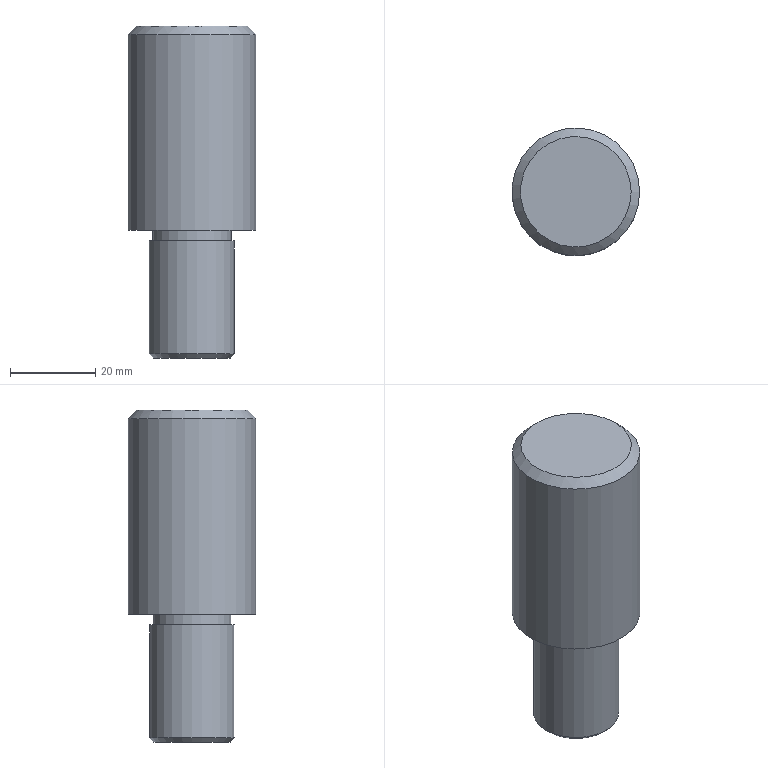Part | NX | features CYLINDER 3, CHAMFER 2, DATUM_CSYS 1 | 1 solid | 9 faces | box 30 x 30 x 78 mm | volume 43030 mm3 | plane 4 | cylinder 3 | cone 2 | commonest cylinder face diameters 18.5 x1 20 x1 30 x1
STEP:
#1=CARTESIAN_POINT('',(13.,0.,48.));
#2=VERTEX_POINT('',#1);
#3=CARTESIAN_POINT('',(0.,0.,48.));
#4=DIRECTION('',(0.,0.,1.));
#5=DIRECTION('',(1.,0.,0.));
#6=AXIS2_PLACEMENT_3D('',#3,#4,#5);
#7=CIRCLE('',#6,13.);
#8=EDGE_CURVE('',#2,#2,#7,.T.);
#9=ORIENTED_EDGE('',*,*,#8,.T.);
#10=EDGE_LOOP('',(#9));
#11=FACE_BOUND('',#10,.T.);
#12=CARTESIAN_POINT('',(0.,0.,48.));
#13=DIRECTION('',(0.,0.,1.));
#14=DIRECTION('',(1.,0.,0.));
#15=AXIS2_PLACEMENT_3D('',#12,#13,#14);
#16=PLANE('',#15);
#17=ADVANCED_FACE('',(#11),#16,.T.);
#18=CARTESIAN_POINT('',(9.25,0.,0.));
#19=VERTEX_POINT('',#18);
#20=CARTESIAN_POINT('',(0.,0.,0.));
#21=DIRECTION('',(0.,0.,-1.));
#22=DIRECTION('',(1.,0.,0.));
#23=AXIS2_PLACEMENT_3D('',#20,#21,#22);
#24=CIRCLE('',#23,9.25);
#25=EDGE_CURVE('',#19,#19,#24,.T.);
#26=ORIENTED_EDGE('',*,*,#25,.F.);
#27=EDGE_LOOP('',(#26));
#28=FACE_BOUND('',#27,.T.);
#29=CARTESIAN_POINT('',(15.,0.,0.));
#30=VERTEX_POINT('',#29);
#31=CARTESIAN_POINT('',(0.,0.,0.));
#32=DIRECTION('',(0.,0.,1.));
#33=DIRECTION('',(1.,0.,0.));
#34=AXIS2_PLACEMENT_3D('',#31,#32,#33);
#35=CIRCLE('',#34,15.);
#36=EDGE_CURVE('',#30,#30,#35,.T.);
#37=ORIENTED_EDGE('',*,*,#36,.F.);
#38=EDGE_LOOP('',(#37));
#39=FACE_BOUND('',#38,.T.);
#40=CARTESIAN_POINT('',(0.,0.,0.));
#41=DIRECTION('',(0.,0.,-1.));
#42=DIRECTION('',(-1.,0.,0.));
#43=AXIS2_PLACEMENT_3D('',#40,#41,#42);
#44=PLANE('',#43);
#45=ADVANCED_FACE('',(#28,#39),#44,.T.);
#46=CARTESIAN_POINT('',(15.,0.,46.));
#47=VERTEX_POINT('',#46);
#48=CARTESIAN_POINT('',(0.,0.,46.));
#49=DIRECTION('',(0.,0.,1.));
#50=DIRECTION('',(1.,0.,0.));
#51=AXIS2_PLACEMENT_3D('',#48,#49,#50);
#52=CIRCLE('',#51,15.);
#53=EDGE_CURVE('',#47,#47,#52,.F.);
#54=ORIENTED_EDGE('',*,*,#53,.T.);
#55=EDGE_LOOP('',(#54));
#56=FACE_BOUND('',#55,.T.);
#57=ORIENTED_EDGE('',*,*,#36,.T.);
#58=EDGE_LOOP('',(#57));
#59=FACE_BOUND('',#58,.T.);
#60=CARTESIAN_POINT('',(0.,0.,0.));
#61=DIRECTION('',(0.,0.,1.));
#62=DIRECTION('',(1.,0.,0.));
#63=AXIS2_PLACEMENT_3D('',#60,#61,#62);
#64=CYLINDRICAL_SURFACE('',#63,15.);
#65=ADVANCED_FACE('',(#56,#59),#64,.T.);
#66=CARTESIAN_POINT('',(9.25,0.,-2.5));
#67=VERTEX_POINT('',#66);
#68=CARTESIAN_POINT('',(0.,0.,-2.5));
#69=DIRECTION('',(0.,0.,1.));
#70=DIRECTION('',(1.,0.,0.));
#71=AXIS2_PLACEMENT_3D('',#68,#69,#70);
#72=CIRCLE('',#71,9.25);
#73=EDGE_CURVE('',#67,#67,#72,.T.);
#74=ORIENTED_EDGE('',*,*,#73,.T.);
#75=EDGE_LOOP('',(#74));
#76=FACE_BOUND('',#75,.T.);
#77=ORIENTED_EDGE('',*,*,#25,.T.);
#78=EDGE_LOOP('',(#77));
#79=FACE_BOUND('',#78,.T.);
#80=CARTESIAN_POINT('',(0.,0.,0.));
#81=DIRECTION('',(0.,0.,-1.));
#82=DIRECTION('',(1.,0.,0.));
#83=AXIS2_PLACEMENT_3D('',#80,#81,#82);
#84=CYLINDRICAL_SURFACE('',#83,9.25);
#85=ADVANCED_FACE('',(#76,#79),#84,.T.);
#86=CARTESIAN_POINT('',(-9.,0.,-30.));
#87=VERTEX_POINT('',#86);
#88=CARTESIAN_POINT('',(0.,0.,-30.));
#89=DIRECTION('',(0.,0.,-1.));
#90=DIRECTION('',(-1.,0.,0.));
#91=AXIS2_PLACEMENT_3D('',#88,#89,#90);
#92=CIRCLE('',#91,9.);
#93=EDGE_CURVE('',#87,#87,#92,.T.);
#94=ORIENTED_EDGE('',*,*,#93,.T.);
#95=EDGE_LOOP('',(#94));
#96=FACE_BOUND('',#95,.T.);
#97=CARTESIAN_POINT('',(0.,0.,-30.));
#98=DIRECTION('',(0.,0.,-1.));
#99=DIRECTION('',(-1.,0.,0.));
#100=AXIS2_PLACEMENT_3D('',#97,#98,#99);
#101=PLANE('',#100);
#102=ADVANCED_FACE('',(#96),#101,.T.);
#103=ORIENTED_EDGE('',*,*,#73,.F.);
#104=EDGE_LOOP('',(#103));
#105=FACE_BOUND('',#104,.T.);
#106=CARTESIAN_POINT('',(10.,0.,-2.5));
#107=VERTEX_POINT('',#106);
#108=CARTESIAN_POINT('',(0.,0.,-2.5));
#109=DIRECTION('',(0.,0.,-1.));
#110=DIRECTION('',(1.,0.,0.));
#111=AXIS2_PLACEMENT_3D('',#108,#109,#110);
#112=CIRCLE('',#111,10.);
#113=EDGE_CURVE('',#107,#107,#112,.T.);
#114=ORIENTED_EDGE('',*,*,#113,.F.);
#115=EDGE_LOOP('',(#114));
#116=FACE_BOUND('',#115,.T.);
#117=CARTESIAN_POINT('',(0.,0.,-2.5));
#118=DIRECTION('',(0.,0.,1.));
#119=DIRECTION('',(1.,0.,0.));
#120=AXIS2_PLACEMENT_3D('',#117,#118,#119);
#121=PLANE('',#120);
#122=ADVANCED_FACE('',(#105,#116),#121,.T.);
#123=CARTESIAN_POINT('',(-10.,0.,-29.));
#124=VERTEX_POINT('',#123);
#125=CARTESIAN_POINT('',(0.,0.,-29.));
#126=DIRECTION('',(0.,0.,-1.));
#127=DIRECTION('',(-1.,0.,0.));
#128=AXIS2_PLACEMENT_3D('',#125,#126,#127);
#129=CIRCLE('',#128,10.);
#130=EDGE_CURVE('',#124,#124,#129,.F.);
#131=ORIENTED_EDGE('',*,*,#130,.T.);
#132=EDGE_LOOP('',(#131));
#133=FACE_BOUND('',#132,.T.);
#134=ORIENTED_EDGE('',*,*,#113,.T.);
#135=EDGE_LOOP('',(#134));
#136=FACE_BOUND('',#135,.T.);
#137=CARTESIAN_POINT('',(0.,0.,-2.5));
#138=DIRECTION('',(0.,0.,-1.));
#139=DIRECTION('',(1.,0.,0.));
#140=AXIS2_PLACEMENT_3D('',#137,#138,#139);
#141=CYLINDRICAL_SURFACE('',#140,10.);
#142=ADVANCED_FACE('',(#133,#136),#141,.T.);
#143=ORIENTED_EDGE('',*,*,#8,.F.);
#144=EDGE_LOOP('',(#143));
#145=FACE_BOUND('',#144,.T.);
#146=ORIENTED_EDGE('',*,*,#53,.F.);
#147=EDGE_LOOP('',(#146));
#148=FACE_BOUND('',#147,.T.);
#149=CARTESIAN_POINT('',(0.,0.,46.));
#150=DIRECTION('',(0.,0.,-1.));
#151=DIRECTION('',(-1.,0.,0.));
#152=AXIS2_PLACEMENT_3D('',#149,#150,#151);
#153=CONICAL_SURFACE('',#152,15.,0.7854);
#154=ADVANCED_FACE('',(#145,#148),#153,.T.);
#155=ORIENTED_EDGE('',*,*,#93,.F.);
#156=EDGE_LOOP('',(#155));
#157=FACE_BOUND('',#156,.T.);
#158=ORIENTED_EDGE('',*,*,#130,.F.);
#159=EDGE_LOOP('',(#158));
#160=FACE_BOUND('',#159,.T.);
#161=CARTESIAN_POINT('',(0.,0.,-29.));
#162=DIRECTION('',(0.,0.,1.));
#163=DIRECTION('',(1.,0.,0.));
#164=AXIS2_PLACEMENT_3D('',#161,#162,#163);
#165=CONICAL_SURFACE('',#164,10.,0.7854);
#166=ADVANCED_FACE('',(#157,#160),#165,.T.);
#167=CLOSED_SHELL('',(#17,#45,#65,#85,#102,#122,#142,#154,#166));
#168=MANIFOLD_SOLID_BREP('',#167);
#169=(LENGTH_UNIT()NAMED_UNIT(*)SI_UNIT(.MILLI.,.METRE.));
#170=UNCERTAINTY_MEASURE_WITH_UNIT(LENGTH_MEASURE(0.00001),#169,'','');
#171=(NAMED_UNIT(*)PLANE_ANGLE_UNIT()SI_UNIT($,.RADIAN.));
#172=(NAMED_UNIT(*)SI_UNIT($,.STERADIAN.)SOLID_ANGLE_UNIT());
#173=(GEOMETRIC_REPRESENTATION_CONTEXT(3)GLOBAL_UNCERTAINTY_ASSIGNED_CONTEXT((#170))GLOBAL_UNIT_ASSIGNED_CONTEXT((#169,#171,#172))REPRESENTATION_CONTEXT('',''));
#174=ADVANCED_BREP_SHAPE_REPRESENTATION('',(#168),#173);